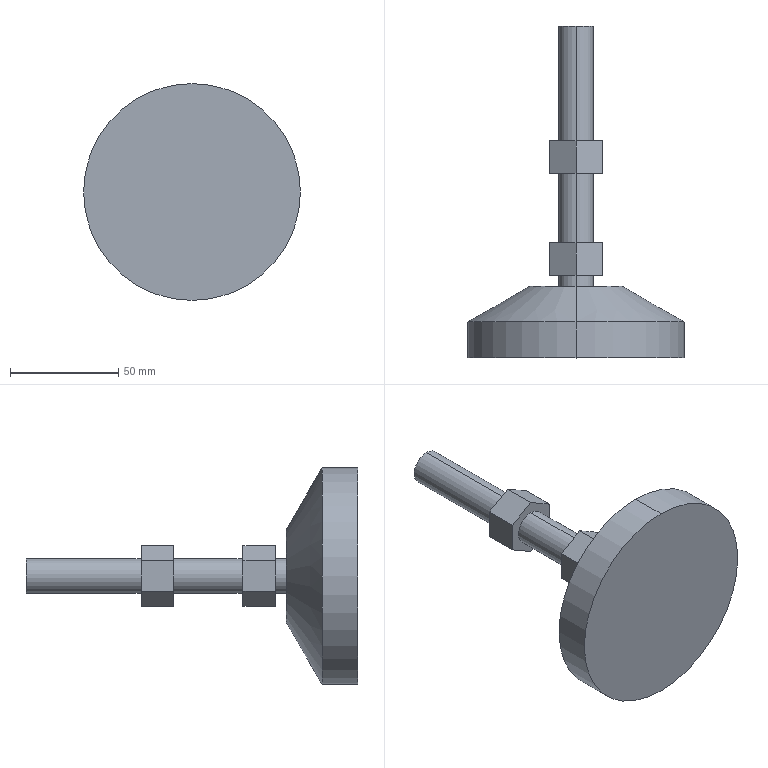Part | SolidWorks | features ICE 3, Revolution 1 | 2 solids | 27 faces | box 100 x 153 x 100 mm | volume 235299 mm3 | plane 19 | cylinder 6 | cone 2 | commonest cylinder face diameters 16 x4 100 x2
STEP:
#1=CARTESIAN_POINT('',(0.,38.,13.856));
#2=VERTEX_POINT('',#1);
#3=CARTESIAN_POINT('',(12.,38.,6.928));
#4=VERTEX_POINT('',#3);
#5=CARTESIAN_POINT('',(0.,38.,13.856));
#6=DIRECTION('',(0.866,0.,-0.5));
#7=VECTOR('',#6,1000.);
#8=LINE('',#5,#7);
#9=EDGE_CURVE('',#2,#4,#8,.T.);
#10=ORIENTED_EDGE('',*,*,#9,.T.);
#11=CARTESIAN_POINT('',(12.,53.,6.928));
#12=VERTEX_POINT('',#11);
#13=CARTESIAN_POINT('',(12.,53.,6.928));
#14=DIRECTION('',(0.,-1.,0.));
#15=VECTOR('',#14,1000.);
#16=LINE('',#13,#15);
#17=EDGE_CURVE('',#12,#4,#16,.T.);
#18=ORIENTED_EDGE('',*,*,#17,.F.);
#19=CARTESIAN_POINT('',(0.,53.,13.856));
#20=VERTEX_POINT('',#19);
#21=CARTESIAN_POINT('',(0.,53.,13.856));
#22=DIRECTION('',(0.866,0.,-0.5));
#23=VECTOR('',#22,1000.);
#24=LINE('',#21,#23);
#25=EDGE_CURVE('',#20,#12,#24,.T.);
#26=ORIENTED_EDGE('',*,*,#25,.F.);
#27=CARTESIAN_POINT('',(0.,53.,13.856));
#28=DIRECTION('',(0.,-1.,0.));
#29=VECTOR('',#28,1000.);
#30=LINE('',#27,#29);
#31=EDGE_CURVE('',#20,#2,#30,.T.);
#32=ORIENTED_EDGE('',*,*,#31,.T.);
#33=EDGE_LOOP('',(#10,#18,#26,#32));
#34=FACE_OUTER_BOUND('',#33,.T.);
#35=CARTESIAN_POINT('',(0.,53.,13.856));
#36=DIRECTION('',(-0.5,0.,-0.866));
#37=DIRECTION('',(-0.866,0.,0.5));
#38=AXIS2_PLACEMENT_3D('',#35,#36,#37);
#39=PLANE('',#38);
#40=ADVANCED_FACE('',(#34),#39,.F.);
#41=CARTESIAN_POINT('',(12.,38.,-6.928));
#42=VERTEX_POINT('',#41);
#43=CARTESIAN_POINT('',(12.,38.,6.928));
#44=DIRECTION('',(0.,0.,-1.));
#45=VECTOR('',#44,1000.);
#46=LINE('',#43,#45);
#47=EDGE_CURVE('',#4,#42,#46,.T.);
#48=ORIENTED_EDGE('',*,*,#47,.T.);
#49=CARTESIAN_POINT('',(12.,53.,-6.928));
#50=VERTEX_POINT('',#49);
#51=CARTESIAN_POINT('',(12.,53.,-6.928));
#52=DIRECTION('',(0.,-1.,0.));
#53=VECTOR('',#52,1000.);
#54=LINE('',#51,#53);
#55=EDGE_CURVE('',#50,#42,#54,.T.);
#56=ORIENTED_EDGE('',*,*,#55,.F.);
#57=CARTESIAN_POINT('',(12.,53.,6.928));
#58=DIRECTION('',(0.,0.,-1.));
#59=VECTOR('',#58,1000.);
#60=LINE('',#57,#59);
#61=EDGE_CURVE('',#12,#50,#60,.T.);
#62=ORIENTED_EDGE('',*,*,#61,.F.);
#63=ORIENTED_EDGE('',*,*,#17,.T.);
#64=EDGE_LOOP('',(#48,#56,#62,#63));
#65=FACE_OUTER_BOUND('',#64,.T.);
#66=CARTESIAN_POINT('',(12.,53.,6.928));
#67=DIRECTION('',(-1.,0.,0.));
#68=DIRECTION('',(0.,0.,1.));
#69=AXIS2_PLACEMENT_3D('',#66,#67,#68);
#70=PLANE('',#69);
#71=ADVANCED_FACE('',(#65),#70,.F.);
#72=CARTESIAN_POINT('',(0.,38.,-13.856));
#73=VERTEX_POINT('',#72);
#74=CARTESIAN_POINT('',(12.,38.,-6.928));
#75=DIRECTION('',(-0.866,0.,-0.5));
#76=VECTOR('',#75,1000.);
#77=LINE('',#74,#76);
#78=EDGE_CURVE('',#42,#73,#77,.T.);
#79=ORIENTED_EDGE('',*,*,#78,.T.);
#80=CARTESIAN_POINT('',(0.,53.,-13.856));
#81=VERTEX_POINT('',#80);
#82=CARTESIAN_POINT('',(0.,53.,-13.856));
#83=DIRECTION('',(0.,-1.,0.));
#84=VECTOR('',#83,1000.);
#85=LINE('',#82,#84);
#86=EDGE_CURVE('',#81,#73,#85,.T.);
#87=ORIENTED_EDGE('',*,*,#86,.F.);
#88=CARTESIAN_POINT('',(12.,53.,-6.928));
#89=DIRECTION('',(-0.866,0.,-0.5));
#90=VECTOR('',#89,1000.);
#91=LINE('',#88,#90);
#92=EDGE_CURVE('',#50,#81,#91,.T.);
#93=ORIENTED_EDGE('',*,*,#92,.F.);
#94=ORIENTED_EDGE('',*,*,#55,.T.);
#95=EDGE_LOOP('',(#79,#87,#93,#94));
#96=FACE_OUTER_BOUND('',#95,.T.);
#97=CARTESIAN_POINT('',(12.,53.,-6.928));
#98=DIRECTION('',(-0.5,0.,0.866));
#99=DIRECTION('',(0.866,0.,0.5));
#100=AXIS2_PLACEMENT_3D('',#97,#98,#99);
#101=PLANE('',#100);
#102=ADVANCED_FACE('',(#96),#101,.F.);
#103=CARTESIAN_POINT('',(-12.,38.,-6.928));
#104=VERTEX_POINT('',#103);
#105=CARTESIAN_POINT('',(0.,38.,-13.856));
#106=DIRECTION('',(-0.866,0.,0.5));
#107=VECTOR('',#106,1000.);
#108=LINE('',#105,#107);
#109=EDGE_CURVE('',#73,#104,#108,.T.);
#110=ORIENTED_EDGE('',*,*,#109,.T.);
#111=CARTESIAN_POINT('',(-12.,53.,-6.928));
#112=VERTEX_POINT('',#111);
#113=CARTESIAN_POINT('',(-12.,53.,-6.928));
#114=DIRECTION('',(0.,-1.,0.));
#115=VECTOR('',#114,1000.);
#116=LINE('',#113,#115);
#117=EDGE_CURVE('',#112,#104,#116,.T.);
#118=ORIENTED_EDGE('',*,*,#117,.F.);
#119=CARTESIAN_POINT('',(0.,53.,-13.856));
#120=DIRECTION('',(-0.866,0.,0.5));
#121=VECTOR('',#120,1000.);
#122=LINE('',#119,#121);
#123=EDGE_CURVE('',#81,#112,#122,.T.);
#124=ORIENTED_EDGE('',*,*,#123,.F.);
#125=ORIENTED_EDGE('',*,*,#86,.T.);
#126=EDGE_LOOP('',(#110,#118,#124,#125));
#127=FACE_OUTER_BOUND('',#126,.T.);
#128=CARTESIAN_POINT('',(0.,53.,-13.856));
#129=DIRECTION('',(0.5,0.,0.866));
#130=DIRECTION('',(0.866,0.,-0.5));
#131=AXIS2_PLACEMENT_3D('',#128,#129,#130);
#132=PLANE('',#131);
#133=ADVANCED_FACE('',(#127),#132,.F.);
#134=CARTESIAN_POINT('',(-12.,38.,6.928));
#135=VERTEX_POINT('',#134);
#136=CARTESIAN_POINT('',(-12.,38.,-6.928));
#137=DIRECTION('',(0.,0.,1.));
#138=VECTOR('',#137,1000.);
#139=LINE('',#136,#138);
#140=EDGE_CURVE('',#104,#135,#139,.T.);
#141=ORIENTED_EDGE('',*,*,#140,.T.);
#142=CARTESIAN_POINT('',(-12.,53.,6.928));
#143=VERTEX_POINT('',#142);
#144=CARTESIAN_POINT('',(-12.,53.,6.928));
#145=DIRECTION('',(0.,-1.,0.));
#146=VECTOR('',#145,1000.);
#147=LINE('',#144,#146);
#148=EDGE_CURVE('',#143,#135,#147,.T.);
#149=ORIENTED_EDGE('',*,*,#148,.F.);
#150=CARTESIAN_POINT('',(-12.,53.,-6.928));
#151=DIRECTION('',(0.,0.,1.));
#152=VECTOR('',#151,1000.);
#153=LINE('',#150,#152);
#154=EDGE_CURVE('',#112,#143,#153,.T.);
#155=ORIENTED_EDGE('',*,*,#154,.F.);
#156=ORIENTED_EDGE('',*,*,#117,.T.);
#157=EDGE_LOOP('',(#141,#149,#155,#156));
#158=FACE_OUTER_BOUND('',#157,.T.);
#159=CARTESIAN_POINT('',(-12.,53.,-6.928));
#160=DIRECTION('',(1.,0.,0.));
#161=DIRECTION('',(0.,0.,-1.));
#162=AXIS2_PLACEMENT_3D('',#159,#160,#161);
#163=PLANE('',#162);
#164=ADVANCED_FACE('',(#158),#163,.F.);
#165=CARTESIAN_POINT('',(-12.,38.,6.928));
#166=DIRECTION('',(0.866,0.,0.5));
#167=VECTOR('',#166,1000.);
#168=LINE('',#165,#167);
#169=EDGE_CURVE('',#135,#2,#168,.T.);
#170=ORIENTED_EDGE('',*,*,#169,.T.);
#171=ORIENTED_EDGE('',*,*,#31,.F.);
#172=CARTESIAN_POINT('',(-12.,53.,6.928));
#173=DIRECTION('',(0.866,0.,0.5));
#174=VECTOR('',#173,1000.);
#175=LINE('',#172,#174);
#176=EDGE_CURVE('',#143,#20,#175,.T.);
#177=ORIENTED_EDGE('',*,*,#176,.F.);
#178=ORIENTED_EDGE('',*,*,#148,.T.);
#179=EDGE_LOOP('',(#170,#171,#177,#178));
#180=FACE_OUTER_BOUND('',#179,.T.);
#181=CARTESIAN_POINT('',(-12.,53.,6.928));
#182=DIRECTION('',(0.5,0.,-0.866));
#183=DIRECTION('',(-0.866,0.,-0.5));
#184=AXIS2_PLACEMENT_3D('',#181,#182,#183);
#185=PLANE('',#184);
#186=ADVANCED_FACE('',(#180),#185,.F.);
#187=ORIENTED_EDGE('',*,*,#25,.T.);
#188=ORIENTED_EDGE('',*,*,#61,.T.);
#189=ORIENTED_EDGE('',*,*,#92,.T.);
#190=ORIENTED_EDGE('',*,*,#123,.T.);
#191=ORIENTED_EDGE('',*,*,#154,.T.);
#192=ORIENTED_EDGE('',*,*,#176,.T.);
#193=EDGE_LOOP('',(#187,#188,#189,#190,#191,#192));
#194=FACE_OUTER_BOUND('',#193,.T.);
#195=CARTESIAN_POINT('',(0.,53.,0.));
#196=DIRECTION('',(0.,1.,0.));
#197=DIRECTION('',(0.,0.,1.));
#198=AXIS2_PLACEMENT_3D('',#195,#196,#197);
#199=PLANE('',#198);
#200=ADVANCED_FACE('',(#194),#199,.T.);
#201=ORIENTED_EDGE('',*,*,#9,.F.);
#202=ORIENTED_EDGE('',*,*,#169,.F.);
#203=ORIENTED_EDGE('',*,*,#140,.F.);
#204=ORIENTED_EDGE('',*,*,#109,.F.);
#205=ORIENTED_EDGE('',*,*,#78,.F.);
#206=ORIENTED_EDGE('',*,*,#47,.F.);
#207=EDGE_LOOP('',(#201,#202,#203,#204,#205,#206));
#208=FACE_OUTER_BOUND('',#207,.T.);
#209=CARTESIAN_POINT('',(0.,38.,0.));
#210=DIRECTION('',(0.,1.,0.));
#211=DIRECTION('',(0.,0.,1.));
#212=AXIS2_PLACEMENT_3D('',#209,#210,#211);
#213=PLANE('',#212);
#214=ADVANCED_FACE('',(#208),#213,.F.);
#215=CLOSED_SHELL('',(#40,#71,#102,#133,#164,#186,#200,#214));
#216=MANIFOLD_SOLID_BREP('',#215);
#217=CARTESIAN_POINT('',(0.,100.,-8.));
#218=VERTEX_POINT('',#217);
#219=CARTESIAN_POINT('',(0.,100.,8.));
#220=VERTEX_POINT('',#219);
#221=CARTESIAN_POINT('',(0.,100.,0.));
#222=DIRECTION('',(0.,-1.,0.));
#223=DIRECTION('',(0.,0.,1.));
#224=AXIS2_PLACEMENT_3D('',#221,#222,#223);
#225=CIRCLE('',#224,8.);
#226=EDGE_CURVE('',#218,#220,#225,.T.);
#227=ORIENTED_EDGE('',*,*,#226,.F.);
#228=CARTESIAN_POINT('',(0.,153.,-8.));
#229=VERTEX_POINT('',#228);
#230=CARTESIAN_POINT('',(0.,10.373,-8.));
#231=DIRECTION('',(0.,1.,0.));
#232=VECTOR('',#231,1000.);
#233=LINE('',#230,#232);
#234=EDGE_CURVE('',#218,#229,#233,.T.);
#235=ORIENTED_EDGE('',*,*,#234,.T.);
#236=CARTESIAN_POINT('',(0.,153.,8.));
#237=VERTEX_POINT('',#236);
#238=CARTESIAN_POINT('',(0.,153.,0.));
#239=DIRECTION('',(0.,1.,0.));
#240=DIRECTION('',(0.,0.,1.));
#241=AXIS2_PLACEMENT_3D('',#238,#239,#240);
#242=CIRCLE('',#241,8.);
#243=EDGE_CURVE('',#237,#229,#242,.T.);
#244=ORIENTED_EDGE('',*,*,#243,.F.);
#245=CARTESIAN_POINT('',(0.,10.373,8.));
#246=DIRECTION('',(0.,1.,0.));
#247=VECTOR('',#246,1000.);
#248=LINE('',#245,#247);
#249=EDGE_CURVE('',#220,#237,#248,.T.);
#250=ORIENTED_EDGE('',*,*,#249,.F.);
#251=EDGE_LOOP('',(#227,#235,#244,#250));
#252=FACE_OUTER_BOUND('',#251,.T.);
#253=CARTESIAN_POINT('',(0.,10.373,0.));
#254=DIRECTION('',(0.,1.,0.));
#255=DIRECTION('',(0.,0.,1.));
#256=AXIS2_PLACEMENT_3D('',#253,#254,#255);
#257=CYLINDRICAL_SURFACE('',#256,8.);
#258=ADVANCED_FACE('',(#252),#257,.T.);
#259=CARTESIAN_POINT('',(0.,33.,-21.421));
#260=VERTEX_POINT('',#259);
#261=CARTESIAN_POINT('',(0.,33.,21.421));
#262=VERTEX_POINT('',#261);
#263=CARTESIAN_POINT('',(0.,33.,0.));
#264=DIRECTION('',(0.,-1.,0.));
#265=DIRECTION('',(0.,0.,-1.));
#266=AXIS2_PLACEMENT_3D('',#263,#264,#265);
#267=CIRCLE('',#266,21.421);
#268=EDGE_CURVE('',#260,#262,#267,.T.);
#269=ORIENTED_EDGE('',*,*,#268,.T.);
#270=CARTESIAN_POINT('',(0.,16.5,50.));
#271=VERTEX_POINT('',#270);
#272=CARTESIAN_POINT('',(0.,16.5,50.));
#273=DIRECTION('',(0.,-0.5,0.866));
#274=VECTOR('',#273,1000.);
#275=LINE('',#272,#274);
#276=EDGE_CURVE('',#262,#271,#275,.T.);
#277=ORIENTED_EDGE('',*,*,#276,.T.);
#278=CARTESIAN_POINT('',(0.,16.5,-50.));
#279=VERTEX_POINT('',#278);
#280=CARTESIAN_POINT('',(0.,16.5,0.));
#281=DIRECTION('',(0.,-1.,0.));
#282=DIRECTION('',(0.,0.,-1.));
#283=AXIS2_PLACEMENT_3D('',#280,#281,#282);
#284=CIRCLE('',#283,50.);
#285=EDGE_CURVE('',#279,#271,#284,.T.);
#286=ORIENTED_EDGE('',*,*,#285,.F.);
#287=CARTESIAN_POINT('',(0.,16.5,-50.));
#288=DIRECTION('',(0.,-0.5,-0.866));
#289=VECTOR('',#288,1000.);
#290=LINE('',#287,#289);
#291=EDGE_CURVE('',#260,#279,#290,.T.);
#292=ORIENTED_EDGE('',*,*,#291,.F.);
#293=EDGE_LOOP('',(#269,#277,#286,#292));
#294=FACE_OUTER_BOUND('',#293,.T.);
#295=CARTESIAN_POINT('',(0.,16.5,0.));
#296=DIRECTION('',(0.,-1.,0.));
#297=DIRECTION('',(0.,0.,-1.));
#298=AXIS2_PLACEMENT_3D('',#295,#296,#297);
#299=CONICAL_SURFACE('',#298,50.,1.047);
#300=ADVANCED_FACE('',(#294),#299,.T.);
#301=ORIENTED_EDGE('',*,*,#285,.T.);
#302=CARTESIAN_POINT('',(0.,0.,50.));
#303=VERTEX_POINT('',#302);
#304=CARTESIAN_POINT('',(0.,0.,50.));
#305=DIRECTION('',(0.,-1.,0.));
#306=VECTOR('',#305,1000.);
#307=LINE('',#304,#306);
#308=EDGE_CURVE('',#271,#303,#307,.T.);
#309=ORIENTED_EDGE('',*,*,#308,.T.);
#310=CARTESIAN_POINT('',(0.,0.,-50.));
#311=VERTEX_POINT('',#310);
#312=CARTESIAN_POINT('',(0.,0.,0.));
#313=DIRECTION('',(0.,-1.,0.));
#314=DIRECTION('',(0.,0.,-1.));
#315=AXIS2_PLACEMENT_3D('',#312,#313,#314);
#316=CIRCLE('',#315,50.);
#317=EDGE_CURVE('',#311,#303,#316,.T.);
#318=ORIENTED_EDGE('',*,*,#317,.F.);
#319=CARTESIAN_POINT('',(0.,0.,-50.));
#320=DIRECTION('',(0.,-1.,0.));
#321=VECTOR('',#320,1000.);
#322=LINE('',#319,#321);
#323=EDGE_CURVE('',#279,#311,#322,.T.);
#324=ORIENTED_EDGE('',*,*,#323,.F.);
#325=EDGE_LOOP('',(#301,#309,#318,#324));
#326=FACE_OUTER_BOUND('',#325,.T.);
#327=CARTESIAN_POINT('',(0.,0.,0.));
#328=DIRECTION('',(0.,-1.,0.));
#329=DIRECTION('',(0.,0.,-1.));
#330=AXIS2_PLACEMENT_3D('',#327,#328,#329);
#331=CYLINDRICAL_SURFACE('',#330,50.);
#332=ADVANCED_FACE('',(#326),#331,.T.);
#333=CARTESIAN_POINT('',(0.,33.,8.));
#334=VERTEX_POINT('',#333);
#335=CARTESIAN_POINT('',(0.,33.,-8.));
#336=VERTEX_POINT('',#335);
#337=CARTESIAN_POINT('',(0.,33.,0.));
#338=DIRECTION('',(0.,1.,0.));
#339=DIRECTION('',(0.,0.,1.));
#340=AXIS2_PLACEMENT_3D('',#337,#338,#339);
#341=CIRCLE('',#340,8.);
#342=EDGE_CURVE('',#334,#336,#341,.T.);
#343=ORIENTED_EDGE('',*,*,#342,.T.);
#344=CARTESIAN_POINT('',(0.,85.,-8.));
#345=VERTEX_POINT('',#344);
#346=CARTESIAN_POINT('',(0.,10.373,-8.));
#347=DIRECTION('',(0.,1.,0.));
#348=VECTOR('',#347,1000.);
#349=LINE('',#346,#348);
#350=EDGE_CURVE('',#336,#345,#349,.T.);
#351=ORIENTED_EDGE('',*,*,#350,.T.);
#352=CARTESIAN_POINT('',(0.,85.,8.));
#353=VERTEX_POINT('',#352);
#354=CARTESIAN_POINT('',(0.,85.,0.));
#355=DIRECTION('',(0.,-1.,0.));
#356=DIRECTION('',(0.,0.,1.));
#357=AXIS2_PLACEMENT_3D('',#354,#355,#356);
#358=CIRCLE('',#357,8.);
#359=EDGE_CURVE('',#345,#353,#358,.T.);
#360=ORIENTED_EDGE('',*,*,#359,.T.);
#361=CARTESIAN_POINT('',(0.,10.373,8.));
#362=DIRECTION('',(0.,1.,0.));
#363=VECTOR('',#362,1000.);
#364=LINE('',#361,#363);
#365=EDGE_CURVE('',#334,#353,#364,.T.);
#366=ORIENTED_EDGE('',*,*,#365,.F.);
#367=EDGE_LOOP('',(#343,#351,#360,#366));
#368=FACE_OUTER_BOUND('',#367,.T.);
#369=CARTESIAN_POINT('',(0.,10.373,0.));
#370=DIRECTION('',(0.,1.,0.));
#371=DIRECTION('',(0.,0.,1.));
#372=AXIS2_PLACEMENT_3D('',#369,#370,#371);
#373=CYLINDRICAL_SURFACE('',#372,8.);
#374=ADVANCED_FACE('',(#368),#373,.T.);
#375=ORIENTED_EDGE('',*,*,#350,.F.);
#376=CARTESIAN_POINT('',(0.,33.,0.));
#377=DIRECTION('',(0.,1.,0.));
#378=DIRECTION('',(0.,0.,1.));
#379=AXIS2_PLACEMENT_3D('',#376,#377,#378);
#380=CIRCLE('',#379,8.);
#381=EDGE_CURVE('',#336,#334,#380,.T.);
#382=ORIENTED_EDGE('',*,*,#381,.T.);
#383=ORIENTED_EDGE('',*,*,#365,.T.);
#384=CARTESIAN_POINT('',(0.,85.,0.));
#385=DIRECTION('',(0.,-1.,0.));
#386=DIRECTION('',(0.,0.,1.));
#387=AXIS2_PLACEMENT_3D('',#384,#385,#386);
#388=CIRCLE('',#387,8.);
#389=EDGE_CURVE('',#353,#345,#388,.T.);
#390=ORIENTED_EDGE('',*,*,#389,.T.);
#391=EDGE_LOOP('',(#375,#382,#383,#390));
#392=FACE_OUTER_BOUND('',#391,.T.);
#393=CARTESIAN_POINT('',(0.,10.373,0.));
#394=DIRECTION('',(0.,1.,0.));
#395=DIRECTION('',(0.,0.,1.));
#396=AXIS2_PLACEMENT_3D('',#393,#394,#395);
#397=CYLINDRICAL_SURFACE('',#396,8.);
#398=ADVANCED_FACE('',(#392),#397,.T.);
#399=ORIENTED_EDGE('',*,*,#317,.T.);
#400=CARTESIAN_POINT('',(0.,0.,0.));
#401=DIRECTION('',(0.,-1.,0.));
#402=DIRECTION('',(0.,0.,-1.));
#403=AXIS2_PLACEMENT_3D('',#400,#401,#402);
#404=CIRCLE('',#403,50.);
#405=EDGE_CURVE('',#303,#311,#404,.T.);
#406=ORIENTED_EDGE('',*,*,#405,.T.);
#407=EDGE_LOOP('',(#399,#406));
#408=FACE_OUTER_BOUND('',#407,.T.);
#409=CARTESIAN_POINT('',(0.,0.,0.));
#410=DIRECTION('',(0.,-1.,0.));
#411=DIRECTION('',(0.,0.,-1.));
#412=AXIS2_PLACEMENT_3D('',#409,#410,#411);
#413=PLANE('',#412);
#414=ADVANCED_FACE('',(#408),#413,.T.);
#415=ORIENTED_EDGE('',*,*,#308,.F.);
#416=CARTESIAN_POINT('',(0.,16.5,0.));
#417=DIRECTION('',(0.,-1.,0.));
#418=DIRECTION('',(0.,0.,-1.));
#419=AXIS2_PLACEMENT_3D('',#416,#417,#418);
#420=CIRCLE('',#419,50.);
#421=EDGE_CURVE('',#271,#279,#420,.T.);
#422=ORIENTED_EDGE('',*,*,#421,.T.);
#423=ORIENTED_EDGE('',*,*,#323,.T.);
#424=ORIENTED_EDGE('',*,*,#405,.F.);
#425=EDGE_LOOP('',(#415,#422,#423,#424));
#426=FACE_OUTER_BOUND('',#425,.T.);
#427=CARTESIAN_POINT('',(0.,0.,0.));
#428=DIRECTION('',(0.,-1.,0.));
#429=DIRECTION('',(0.,0.,-1.));
#430=AXIS2_PLACEMENT_3D('',#427,#428,#429);
#431=CYLINDRICAL_SURFACE('',#430,50.);
#432=ADVANCED_FACE('',(#426),#431,.T.);
#433=ORIENTED_EDGE('',*,*,#276,.F.);
#434=CARTESIAN_POINT('',(0.,33.,0.));
#435=DIRECTION('',(0.,-1.,0.));
#436=DIRECTION('',(0.,0.,-1.));
#437=AXIS2_PLACEMENT_3D('',#434,#435,#436);
#438=CIRCLE('',#437,21.421);
#439=EDGE_CURVE('',#262,#260,#438,.T.);
#440=ORIENTED_EDGE('',*,*,#439,.T.);
#441=ORIENTED_EDGE('',*,*,#291,.T.);
#442=ORIENTED_EDGE('',*,*,#421,.F.);
#443=EDGE_LOOP('',(#433,#440,#441,#442));
#444=FACE_OUTER_BOUND('',#443,.T.);
#445=CARTESIAN_POINT('',(0.,16.5,0.));
#446=DIRECTION('',(0.,-1.,0.));
#447=DIRECTION('',(0.,0.,-1.));
#448=AXIS2_PLACEMENT_3D('',#445,#446,#447);
#449=CONICAL_SURFACE('',#448,50.,1.047);
#450=ADVANCED_FACE('',(#444),#449,.T.);
#451=ORIENTED_EDGE('',*,*,#342,.F.);
#452=ORIENTED_EDGE('',*,*,#381,.F.);
#453=EDGE_LOOP('',(#451,#452));
#454=FACE_BOUND('',#453,.T.);
#455=ORIENTED_EDGE('',*,*,#268,.F.);
#456=ORIENTED_EDGE('',*,*,#439,.F.);
#457=EDGE_LOOP('',(#455,#456));
#458=FACE_OUTER_BOUND('',#457,.T.);
#459=CARTESIAN_POINT('',(21.421,33.,0.));
#460=DIRECTION('',(0.,1.,0.));
#461=DIRECTION('',(0.,0.,1.));
#462=AXIS2_PLACEMENT_3D('',#459,#460,#461);
#463=PLANE('',#462);
#464=ADVANCED_FACE('',(#454,#458),#463,.T.);
#465=CARTESIAN_POINT('',(-12.,100.,6.928));
#466=VERTEX_POINT('',#465);
#467=CARTESIAN_POINT('',(0.,100.,13.856));
#468=VERTEX_POINT('',#467);
#469=CARTESIAN_POINT('',(-12.,100.,6.928));
#470=DIRECTION('',(0.866,0.,0.5));
#471=VECTOR('',#470,1000.);
#472=LINE('',#469,#471);
#473=EDGE_CURVE('',#466,#468,#472,.T.);
#474=ORIENTED_EDGE('',*,*,#473,.F.);
#475=CARTESIAN_POINT('',(-12.,85.,6.928));
#476=VERTEX_POINT('',#475);
#477=CARTESIAN_POINT('',(-12.,85.,6.928));
#478=DIRECTION('',(0.,1.,0.));
#479=VECTOR('',#478,1000.);
#480=LINE('',#477,#479);
#481=EDGE_CURVE('',#476,#466,#480,.T.);
#482=ORIENTED_EDGE('',*,*,#481,.F.);
#483=CARTESIAN_POINT('',(0.,85.,13.856));
#484=VERTEX_POINT('',#483);
#485=CARTESIAN_POINT('',(-12.,85.,6.928));
#486=DIRECTION('',(0.866,0.,0.5));
#487=VECTOR('',#486,1000.);
#488=LINE('',#485,#487);
#489=EDGE_CURVE('',#476,#484,#488,.T.);
#490=ORIENTED_EDGE('',*,*,#489,.T.);
#491=CARTESIAN_POINT('',(0.,85.,13.856));
#492=DIRECTION('',(0.,1.,0.));
#493=VECTOR('',#492,1000.);
#494=LINE('',#491,#493);
#495=EDGE_CURVE('',#484,#468,#494,.T.);
#496=ORIENTED_EDGE('',*,*,#495,.T.);
#497=EDGE_LOOP('',(#474,#482,#490,#496));
#498=FACE_OUTER_BOUND('',#497,.T.);
#499=CARTESIAN_POINT('',(-12.,85.,6.928));
#500=DIRECTION('',(-0.5,0.,0.866));
#501=DIRECTION('',(0.866,0.,0.5));
#502=AXIS2_PLACEMENT_3D('',#499,#500,#501);
#503=PLANE('',#502);
#504=ADVANCED_FACE('',(#498),#503,.T.);
#505=CARTESIAN_POINT('',(-12.,100.,-6.928));
#506=VERTEX_POINT('',#505);
#507=CARTESIAN_POINT('',(-12.,100.,-6.928));
#508=DIRECTION('',(0.,0.,1.));
#509=VECTOR('',#508,1000.);
#510=LINE('',#507,#509);
#511=EDGE_CURVE('',#506,#466,#510,.T.);
#512=ORIENTED_EDGE('',*,*,#511,.F.);
#513=CARTESIAN_POINT('',(-12.,85.,-6.928));
#514=VERTEX_POINT('',#513);
#515=CARTESIAN_POINT('',(-12.,85.,-6.928));
#516=DIRECTION('',(0.,1.,0.));
#517=VECTOR('',#516,1000.);
#518=LINE('',#515,#517);
#519=EDGE_CURVE('',#514,#506,#518,.T.);
#520=ORIENTED_EDGE('',*,*,#519,.F.);
#521=CARTESIAN_POINT('',(-12.,85.,-6.928));
#522=DIRECTION('',(0.,0.,1.));
#523=VECTOR('',#522,1000.);
#524=LINE('',#521,#523);
#525=EDGE_CURVE('',#514,#476,#524,.T.);
#526=ORIENTED_EDGE('',*,*,#525,.T.);
#527=ORIENTED_EDGE('',*,*,#481,.T.);
#528=EDGE_LOOP('',(#512,#520,#526,#527));
#529=FACE_OUTER_BOUND('',#528,.T.);
#530=CARTESIAN_POINT('',(-12.,85.,-6.928));
#531=DIRECTION('',(-1.,0.,0.));
#532=DIRECTION('',(0.,0.,1.));
#533=AXIS2_PLACEMENT_3D('',#530,#531,#532);
#534=PLANE('',#533);
#535=ADVANCED_FACE('',(#529),#534,.T.);
#536=CARTESIAN_POINT('',(0.,100.,-13.856));
#537=VERTEX_POINT('',#536);
#538=CARTESIAN_POINT('',(0.,100.,-13.856));
#539=DIRECTION('',(-0.866,0.,0.5));
#540=VECTOR('',#539,1000.);
#541=LINE('',#538,#540);
#542=EDGE_CURVE('',#537,#506,#541,.T.);
#543=ORIENTED_EDGE('',*,*,#542,.F.);
#544=CARTESIAN_POINT('',(0.,85.,-13.856));
#545=VERTEX_POINT('',#544);
#546=CARTESIAN_POINT('',(0.,85.,-13.856));
#547=DIRECTION('',(0.,1.,0.));
#548=VECTOR('',#547,1000.);
#549=LINE('',#546,#548);
#550=EDGE_CURVE('',#545,#537,#549,.T.);
#551=ORIENTED_EDGE('',*,*,#550,.F.);
#552=CARTESIAN_POINT('',(0.,85.,-13.856));
#553=DIRECTION('',(-0.866,0.,0.5));
#554=VECTOR('',#553,1000.);
#555=LINE('',#552,#554);
#556=EDGE_CURVE('',#545,#514,#555,.T.);
#557=ORIENTED_EDGE('',*,*,#556,.T.);
#558=ORIENTED_EDGE('',*,*,#519,.T.);
#559=EDGE_LOOP('',(#543,#551,#557,#558));
#560=FACE_OUTER_BOUND('',#559,.T.);
#561=CARTESIAN_POINT('',(0.,85.,-13.856));
#562=DIRECTION('',(-0.5,0.,-0.866));
#563=DIRECTION('',(-0.866,0.,0.5));
#564=AXIS2_PLACEMENT_3D('',#561,#562,#563);
#565=PLANE('',#564);
#566=ADVANCED_FACE('',(#560),#565,.T.);
#567=CARTESIAN_POINT('',(12.,100.,-6.928));
#568=VERTEX_POINT('',#567);
#569=CARTESIAN_POINT('',(12.,100.,-6.928));
#570=DIRECTION('',(-0.866,0.,-0.5));
#571=VECTOR('',#570,1000.);
#572=LINE('',#569,#571);
#573=EDGE_CURVE('',#568,#537,#572,.T.);
#574=ORIENTED_EDGE('',*,*,#573,.F.);
#575=CARTESIAN_POINT('',(12.,85.,-6.928));
#576=VERTEX_POINT('',#575);
#577=CARTESIAN_POINT('',(12.,85.,-6.928));
#578=DIRECTION('',(0.,1.,0.));
#579=VECTOR('',#578,1000.);
#580=LINE('',#577,#579);
#581=EDGE_CURVE('',#576,#568,#580,.T.);
#582=ORIENTED_EDGE('',*,*,#581,.F.);
#583=CARTESIAN_POINT('',(12.,85.,-6.928));
#584=DIRECTION('',(-0.866,0.,-0.5));
#585=VECTOR('',#584,1000.);
#586=LINE('',#583,#585);
#587=EDGE_CURVE('',#576,#545,#586,.T.);
#588=ORIENTED_EDGE('',*,*,#587,.T.);
#589=ORIENTED_EDGE('',*,*,#550,.T.);
#590=EDGE_LOOP('',(#574,#582,#588,#589));
#591=FACE_OUTER_BOUND('',#590,.T.);
#592=CARTESIAN_POINT('',(12.,85.,-6.928));
#593=DIRECTION('',(0.5,0.,-0.866));
#594=DIRECTION('',(-0.866,0.,-0.5));
#595=AXIS2_PLACEMENT_3D('',#592,#593,#594);
#596=PLANE('',#595);
#597=ADVANCED_FACE('',(#591),#596,.T.);
#598=CARTESIAN_POINT('',(12.,100.,6.928));
#599=VERTEX_POINT('',#598);
#600=CARTESIAN_POINT('',(12.,100.,6.928));
#601=DIRECTION('',(0.,0.,-1.));
#602=VECTOR('',#601,1000.);
#603=LINE('',#600,#602);
#604=EDGE_CURVE('',#599,#568,#603,.T.);
#605=ORIENTED_EDGE('',*,*,#604,.F.);
#606=CARTESIAN_POINT('',(12.,85.,6.928));
#607=VERTEX_POINT('',#606);
#608=CARTESIAN_POINT('',(12.,85.,6.928));
#609=DIRECTION('',(0.,1.,0.));
#610=VECTOR('',#609,1000.);
#611=LINE('',#608,#610);
#612=EDGE_CURVE('',#607,#599,#611,.T.);
#613=ORIENTED_EDGE('',*,*,#612,.F.);
#614=CARTESIAN_POINT('',(12.,85.,6.928));
#615=DIRECTION('',(0.,0.,-1.));
#616=VECTOR('',#615,1000.);
#617=LINE('',#614,#616);
#618=EDGE_CURVE('',#607,#576,#617,.T.);
#619=ORIENTED_EDGE('',*,*,#618,.T.);
#620=ORIENTED_EDGE('',*,*,#581,.T.);
#621=EDGE_LOOP('',(#605,#613,#619,#620));
#622=FACE_OUTER_BOUND('',#621,.T.);
#623=CARTESIAN_POINT('',(12.,85.,6.928));
#624=DIRECTION('',(1.,0.,0.));
#625=DIRECTION('',(0.,0.,-1.));
#626=AXIS2_PLACEMENT_3D('',#623,#624,#625);
#627=PLANE('',#626);
#628=ADVANCED_FACE('',(#622),#627,.T.);
#629=CARTESIAN_POINT('',(0.,100.,13.856));
#630=DIRECTION('',(0.866,0.,-0.5));
#631=VECTOR('',#630,1000.);
#632=LINE('',#629,#631);
#633=EDGE_CURVE('',#468,#599,#632,.T.);
#634=ORIENTED_EDGE('',*,*,#633,.F.);
#635=ORIENTED_EDGE('',*,*,#495,.F.);
#636=CARTESIAN_POINT('',(0.,85.,13.856));
#637=DIRECTION('',(0.866,0.,-0.5));
#638=VECTOR('',#637,1000.);
#639=LINE('',#636,#638);
#640=EDGE_CURVE('',#484,#607,#639,.T.);
#641=ORIENTED_EDGE('',*,*,#640,.T.);
#642=ORIENTED_EDGE('',*,*,#612,.T.);
#643=EDGE_LOOP('',(#634,#635,#641,#642));
#644=FACE_OUTER_BOUND('',#643,.T.);
#645=CARTESIAN_POINT('',(0.,85.,13.856));
#646=DIRECTION('',(0.5,0.,0.866));
#647=DIRECTION('',(0.866,0.,-0.5));
#648=AXIS2_PLACEMENT_3D('',#645,#646,#647);
#649=PLANE('',#648);
#650=ADVANCED_FACE('',(#644),#649,.T.);
#651=ORIENTED_EDGE('',*,*,#389,.F.);
#652=ORIENTED_EDGE('',*,*,#359,.F.);
#653=EDGE_LOOP('',(#651,#652));
#654=FACE_BOUND('',#653,.T.);
#655=ORIENTED_EDGE('',*,*,#489,.F.);
#656=ORIENTED_EDGE('',*,*,#525,.F.);
#657=ORIENTED_EDGE('',*,*,#556,.F.);
#658=ORIENTED_EDGE('',*,*,#587,.F.);
#659=ORIENTED_EDGE('',*,*,#618,.F.);
#660=ORIENTED_EDGE('',*,*,#640,.F.);
#661=EDGE_LOOP('',(#655,#656,#657,#658,#659,#660));
#662=FACE_OUTER_BOUND('',#661,.T.);
#663=CARTESIAN_POINT('',(0.,85.,0.));
#664=DIRECTION('',(0.,1.,0.));
#665=DIRECTION('',(0.,0.,1.));
#666=AXIS2_PLACEMENT_3D('',#663,#664,#665);
#667=PLANE('',#666);
#668=ADVANCED_FACE('',(#654,#662),#667,.F.);
#669=CARTESIAN_POINT('',(0.,100.,0.));
#670=DIRECTION('',(0.,-1.,0.));
#671=DIRECTION('',(0.,0.,1.));
#672=AXIS2_PLACEMENT_3D('',#669,#670,#671);
#673=CIRCLE('',#672,8.);
#674=EDGE_CURVE('',#220,#218,#673,.T.);
#675=ORIENTED_EDGE('',*,*,#674,.T.);
#676=ORIENTED_EDGE('',*,*,#226,.T.);
#677=EDGE_LOOP('',(#675,#676));
#678=FACE_BOUND('',#677,.T.);
#679=ORIENTED_EDGE('',*,*,#473,.T.);
#680=ORIENTED_EDGE('',*,*,#633,.T.);
#681=ORIENTED_EDGE('',*,*,#604,.T.);
#682=ORIENTED_EDGE('',*,*,#573,.T.);
#683=ORIENTED_EDGE('',*,*,#542,.T.);
#684=ORIENTED_EDGE('',*,*,#511,.T.);
#685=EDGE_LOOP('',(#679,#680,#681,#682,#683,#684));
#686=FACE_OUTER_BOUND('',#685,.T.);
#687=CARTESIAN_POINT('',(0.,100.,0.));
#688=DIRECTION('',(0.,1.,0.));
#689=DIRECTION('',(0.,0.,1.));
#690=AXIS2_PLACEMENT_3D('',#687,#688,#689);
#691=PLANE('',#690);
#692=ADVANCED_FACE('',(#678,#686),#691,.T.);
#693=ORIENTED_EDGE('',*,*,#243,.T.);
#694=CARTESIAN_POINT('',(0.,153.,0.));
#695=DIRECTION('',(0.,1.,0.));
#696=DIRECTION('',(0.,0.,1.));
#697=AXIS2_PLACEMENT_3D('',#694,#695,#696);
#698=CIRCLE('',#697,8.);
#699=EDGE_CURVE('',#229,#237,#698,.T.);
#700=ORIENTED_EDGE('',*,*,#699,.T.);
#701=EDGE_LOOP('',(#693,#700));
#702=FACE_OUTER_BOUND('',#701,.T.);
#703=CARTESIAN_POINT('',(0.,153.,0.));
#704=DIRECTION('',(0.,1.,0.));
#705=DIRECTION('',(0.,0.,1.));
#706=AXIS2_PLACEMENT_3D('',#703,#704,#705);
#707=PLANE('',#706);
#708=ADVANCED_FACE('',(#702),#707,.T.);
#709=ORIENTED_EDGE('',*,*,#234,.F.);
#710=ORIENTED_EDGE('',*,*,#674,.F.);
#711=ORIENTED_EDGE('',*,*,#249,.T.);
#712=ORIENTED_EDGE('',*,*,#699,.F.);
#713=EDGE_LOOP('',(#709,#710,#711,#712));
#714=FACE_OUTER_BOUND('',#713,.T.);
#715=CARTESIAN_POINT('',(0.,10.373,0.));
#716=DIRECTION('',(0.,1.,0.));
#717=DIRECTION('',(0.,0.,1.));
#718=AXIS2_PLACEMENT_3D('',#715,#716,#717);
#719=CYLINDRICAL_SURFACE('',#718,8.);
#720=ADVANCED_FACE('',(#714),#719,.T.);
#721=CLOSED_SHELL('',(#258,#300,#332,#374,#398,#414,#432,#450,#464,#504,#535,#566,#597,#628,#650,#668,#692,#708,#720));
#722=MANIFOLD_SOLID_BREP('',#721);
#723=CARTESIAN_POINT('',(0.,0.,0.));
#724=DIRECTION('',(0.,0.,1.));
#725=DIRECTION('',(1.,0.,0.));
#726=AXIS2_PLACEMENT_3D('',#723,#724,#725);
#727=(LENGTH_UNIT()NAMED_UNIT(*)SI_UNIT(.MILLI.,.METRE.));
#728=UNCERTAINTY_MEASURE_WITH_UNIT(LENGTH_MEASURE(0.00001),#727,'','');
#729=(NAMED_UNIT(*)PLANE_ANGLE_UNIT()SI_UNIT($,.RADIAN.));
#730=(NAMED_UNIT(*)SI_UNIT($,.STERADIAN.)SOLID_ANGLE_UNIT());
#731=(GEOMETRIC_REPRESENTATION_CONTEXT(3)GLOBAL_UNCERTAINTY_ASSIGNED_CONTEXT((#728))GLOBAL_UNIT_ASSIGNED_CONTEXT((#727,#729,#730))REPRESENTATION_CONTEXT('',''));
#732=ADVANCED_BREP_SHAPE_REPRESENTATION('',(#216,#722,#726),#731);